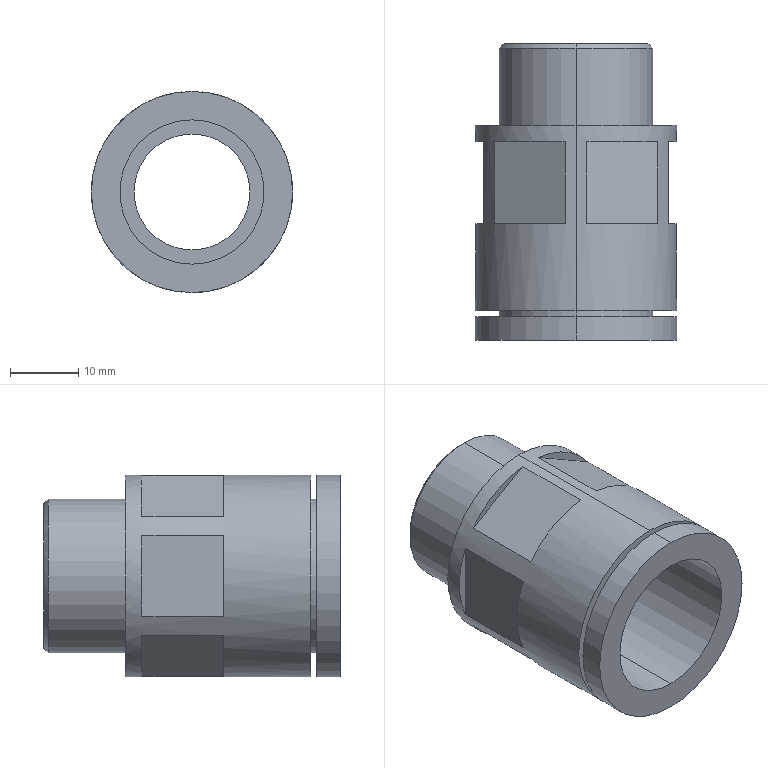Part | STEP file | 00177571_EZT_SCHUTZSCHL.VERS_MKRV-16.5-PG-16.1 | 1 solid | 38 faces | box 29.5 x 43.5 x 29.5 mm | volume 11816 mm3 | plane 24 | cylinder 12 | cone 2 | commonest cylinder face diameters 22.5 x4 29.5 x4 17 x2 21.16 x2